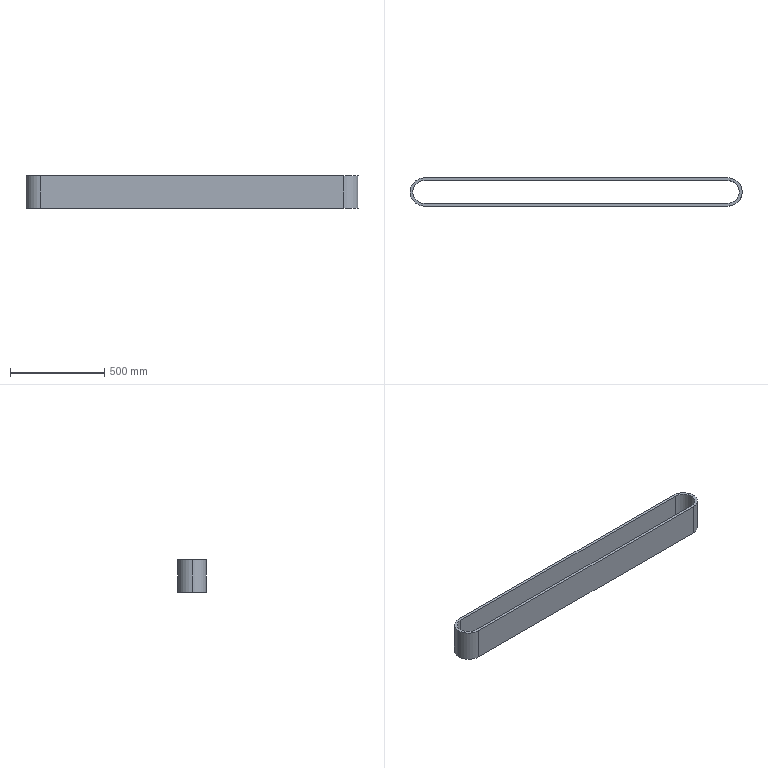Part | SolidWorks | features Extrusion 1 | 1 solid | 12 faces | box 1760 x 150 x 170 mm | volume 9292493 mm3 | cylinder 6 | plane 6 | commonest cylinder face diameters 120 x3 150 x3
STEP:
#1=CARTESIAN_POINT('',(-1610.,60.,170.));
#2=VERTEX_POINT('',#1);
#3=CARTESIAN_POINT('',(-1670.,0.,170.));
#4=VERTEX_POINT('',#3);
#5=CARTESIAN_POINT('',(-1610.,0.,170.));
#6=DIRECTION('',(0.,0.,1.));
#7=DIRECTION('',(1.,0.,0.));
#8=AXIS2_PLACEMENT_3D('',#5,#6,#7);
#9=CIRCLE('',#8,60.);
#10=EDGE_CURVE('',#2,#4,#9,.T.);
#11=ORIENTED_EDGE('',*,*,#10,.T.);
#12=CARTESIAN_POINT('',(-1670.,0.,0.));
#13=VERTEX_POINT('',#12);
#14=CARTESIAN_POINT('',(-1670.,0.,170.));
#15=DIRECTION('',(0.,0.,-1.));
#16=VECTOR('',#15,1000.);
#17=LINE('',#14,#16);
#18=EDGE_CURVE('',#4,#13,#17,.T.);
#19=ORIENTED_EDGE('',*,*,#18,.T.);
#20=CARTESIAN_POINT('',(-1610.,60.,0.));
#21=VERTEX_POINT('',#20);
#22=CARTESIAN_POINT('',(-1610.,0.,0.));
#23=DIRECTION('',(0.,0.,1.));
#24=DIRECTION('',(1.,0.,0.));
#25=AXIS2_PLACEMENT_3D('',#22,#23,#24);
#26=CIRCLE('',#25,60.);
#27=EDGE_CURVE('',#21,#13,#26,.T.);
#28=ORIENTED_EDGE('',*,*,#27,.F.);
#29=CARTESIAN_POINT('',(-1610.,60.,170.));
#30=DIRECTION('',(0.,0.,-1.));
#31=VECTOR('',#30,1000.);
#32=LINE('',#29,#31);
#33=EDGE_CURVE('',#2,#21,#32,.T.);
#34=ORIENTED_EDGE('',*,*,#33,.F.);
#35=EDGE_LOOP('',(#11,#19,#28,#34));
#36=FACE_OUTER_BOUND('',#35,.T.);
#37=CARTESIAN_POINT('',(-1610.,0.,170.));
#38=DIRECTION('',(0.,0.,-1.));
#39=DIRECTION('',(-1.,0.,0.));
#40=AXIS2_PLACEMENT_3D('',#37,#38,#39);
#41=CYLINDRICAL_SURFACE('',#40,60.);
#42=ADVANCED_FACE('',(#36),#41,.F.);
#43=CARTESIAN_POINT('',(-1685.,0.,170.));
#44=VERTEX_POINT('',#43);
#45=CARTESIAN_POINT('',(-1610.,-75.,170.));
#46=VERTEX_POINT('',#45);
#47=CARTESIAN_POINT('',(-1610.,0.,170.));
#48=DIRECTION('',(0.,0.,1.));
#49=DIRECTION('',(1.,0.,0.));
#50=AXIS2_PLACEMENT_3D('',#47,#48,#49);
#51=CIRCLE('',#50,75.);
#52=EDGE_CURVE('',#44,#46,#51,.T.);
#53=ORIENTED_EDGE('',*,*,#52,.F.);
#54=CARTESIAN_POINT('',(-1685.,0.,0.));
#55=VERTEX_POINT('',#54);
#56=CARTESIAN_POINT('',(-1685.,0.,170.));
#57=DIRECTION('',(0.,0.,-1.));
#58=VECTOR('',#57,1000.);
#59=LINE('',#56,#58);
#60=EDGE_CURVE('',#44,#55,#59,.T.);
#61=ORIENTED_EDGE('',*,*,#60,.T.);
#62=CARTESIAN_POINT('',(-1610.,-75.,0.));
#63=VERTEX_POINT('',#62);
#64=CARTESIAN_POINT('',(-1610.,0.,0.));
#65=DIRECTION('',(0.,0.,1.));
#66=DIRECTION('',(1.,0.,0.));
#67=AXIS2_PLACEMENT_3D('',#64,#65,#66);
#68=CIRCLE('',#67,75.);
#69=EDGE_CURVE('',#55,#63,#68,.T.);
#70=ORIENTED_EDGE('',*,*,#69,.T.);
#71=CARTESIAN_POINT('',(-1610.,-75.,170.));
#72=DIRECTION('',(0.,0.,-1.));
#73=VECTOR('',#72,1000.);
#74=LINE('',#71,#73);
#75=EDGE_CURVE('',#46,#63,#74,.T.);
#76=ORIENTED_EDGE('',*,*,#75,.F.);
#77=EDGE_LOOP('',(#53,#61,#70,#76));
#78=FACE_OUTER_BOUND('',#77,.T.);
#79=CARTESIAN_POINT('',(-1610.,0.,170.));
#80=DIRECTION('',(0.,0.,-1.));
#81=DIRECTION('',(-1.,0.,0.));
#82=AXIS2_PLACEMENT_3D('',#79,#80,#81);
#83=CYLINDRICAL_SURFACE('',#82,75.);
#84=ADVANCED_FACE('',(#78),#83,.T.);
#85=CARTESIAN_POINT('',(0.,-75.,170.));
#86=VERTEX_POINT('',#85);
#87=CARTESIAN_POINT('',(0.,75.,170.));
#88=VERTEX_POINT('',#87);
#89=CARTESIAN_POINT('',(0.,0.,170.));
#90=DIRECTION('',(0.,0.,1.));
#91=DIRECTION('',(1.,0.,0.));
#92=AXIS2_PLACEMENT_3D('',#89,#90,#91);
#93=CIRCLE('',#92,75.);
#94=EDGE_CURVE('',#86,#88,#93,.T.);
#95=ORIENTED_EDGE('',*,*,#94,.T.);
#96=CARTESIAN_POINT('',(-1610.,75.,170.));
#97=VERTEX_POINT('',#96);
#98=CARTESIAN_POINT('',(0.,75.,170.));
#99=DIRECTION('',(-1.,0.,0.));
#100=VECTOR('',#99,1000.);
#101=LINE('',#98,#100);
#102=EDGE_CURVE('',#88,#97,#101,.T.);
#103=ORIENTED_EDGE('',*,*,#102,.T.);
#104=CARTESIAN_POINT('',(-1610.,0.,170.));
#105=DIRECTION('',(0.,0.,1.));
#106=DIRECTION('',(1.,0.,0.));
#107=AXIS2_PLACEMENT_3D('',#104,#105,#106);
#108=CIRCLE('',#107,75.);
#109=EDGE_CURVE('',#97,#44,#108,.T.);
#110=ORIENTED_EDGE('',*,*,#109,.T.);
#111=ORIENTED_EDGE('',*,*,#52,.T.);
#112=CARTESIAN_POINT('',(0.,-75.,170.));
#113=DIRECTION('',(1.,0.,0.));
#114=VECTOR('',#113,1000.);
#115=LINE('',#112,#114);
#116=EDGE_CURVE('',#46,#86,#115,.T.);
#117=ORIENTED_EDGE('',*,*,#116,.T.);
#118=EDGE_LOOP('',(#95,#103,#110,#111,#117));
#119=FACE_OUTER_BOUND('',#118,.T.);
#120=CARTESIAN_POINT('',(0.,60.,170.));
#121=VERTEX_POINT('',#120);
#122=CARTESIAN_POINT('',(0.,60.,170.));
#123=DIRECTION('',(-1.,0.,0.));
#124=VECTOR('',#123,1000.);
#125=LINE('',#122,#124);
#126=EDGE_CURVE('',#121,#2,#125,.T.);
#127=ORIENTED_EDGE('',*,*,#126,.F.);
#128=CARTESIAN_POINT('',(0.,-60.,170.));
#129=VERTEX_POINT('',#128);
#130=CARTESIAN_POINT('',(0.,0.,170.));
#131=DIRECTION('',(0.,0.,1.));
#132=DIRECTION('',(1.,0.,0.));
#133=AXIS2_PLACEMENT_3D('',#130,#131,#132);
#134=CIRCLE('',#133,60.);
#135=EDGE_CURVE('',#129,#121,#134,.T.);
#136=ORIENTED_EDGE('',*,*,#135,.F.);
#137=CARTESIAN_POINT('',(-1610.,-60.,170.));
#138=VERTEX_POINT('',#137);
#139=CARTESIAN_POINT('',(0.,-60.,170.));
#140=DIRECTION('',(1.,0.,0.));
#141=VECTOR('',#140,1000.);
#142=LINE('',#139,#141);
#143=EDGE_CURVE('',#138,#129,#142,.T.);
#144=ORIENTED_EDGE('',*,*,#143,.F.);
#145=CARTESIAN_POINT('',(-1610.,0.,170.));
#146=DIRECTION('',(0.,0.,1.));
#147=DIRECTION('',(1.,0.,0.));
#148=AXIS2_PLACEMENT_3D('',#145,#146,#147);
#149=CIRCLE('',#148,60.);
#150=EDGE_CURVE('',#4,#138,#149,.T.);
#151=ORIENTED_EDGE('',*,*,#150,.F.);
#152=ORIENTED_EDGE('',*,*,#10,.F.);
#153=EDGE_LOOP('',(#127,#136,#144,#151,#152));
#154=FACE_BOUND('',#153,.T.);
#155=CARTESIAN_POINT('',(0.,0.,170.));
#156=DIRECTION('',(0.,0.,1.));
#157=DIRECTION('',(1.,0.,0.));
#158=AXIS2_PLACEMENT_3D('',#155,#156,#157);
#159=PLANE('',#158);
#160=ADVANCED_FACE('',(#119,#154),#159,.T.);
#161=CARTESIAN_POINT('',(0.,-75.,0.));
#162=VERTEX_POINT('',#161);
#163=CARTESIAN_POINT('',(0.,75.,0.));
#164=VERTEX_POINT('',#163);
#165=CARTESIAN_POINT('',(0.,0.,0.));
#166=DIRECTION('',(0.,0.,1.));
#167=DIRECTION('',(1.,0.,0.));
#168=AXIS2_PLACEMENT_3D('',#165,#166,#167);
#169=CIRCLE('',#168,75.);
#170=EDGE_CURVE('',#162,#164,#169,.T.);
#171=ORIENTED_EDGE('',*,*,#170,.F.);
#172=CARTESIAN_POINT('',(0.,-75.,0.));
#173=DIRECTION('',(1.,0.,0.));
#174=VECTOR('',#173,1000.);
#175=LINE('',#172,#174);
#176=EDGE_CURVE('',#63,#162,#175,.T.);
#177=ORIENTED_EDGE('',*,*,#176,.F.);
#178=ORIENTED_EDGE('',*,*,#69,.F.);
#179=CARTESIAN_POINT('',(-1610.,75.,0.));
#180=VERTEX_POINT('',#179);
#181=CARTESIAN_POINT('',(-1610.,0.,0.));
#182=DIRECTION('',(0.,0.,1.));
#183=DIRECTION('',(1.,0.,0.));
#184=AXIS2_PLACEMENT_3D('',#181,#182,#183);
#185=CIRCLE('',#184,75.);
#186=EDGE_CURVE('',#180,#55,#185,.T.);
#187=ORIENTED_EDGE('',*,*,#186,.F.);
#188=CARTESIAN_POINT('',(0.,75.,0.));
#189=DIRECTION('',(-1.,0.,0.));
#190=VECTOR('',#189,1000.);
#191=LINE('',#188,#190);
#192=EDGE_CURVE('',#164,#180,#191,.T.);
#193=ORIENTED_EDGE('',*,*,#192,.F.);
#194=EDGE_LOOP('',(#171,#177,#178,#187,#193));
#195=FACE_OUTER_BOUND('',#194,.T.);
#196=CARTESIAN_POINT('',(0.,-60.,0.));
#197=VERTEX_POINT('',#196);
#198=CARTESIAN_POINT('',(0.,60.,0.));
#199=VERTEX_POINT('',#198);
#200=CARTESIAN_POINT('',(0.,0.,0.));
#201=DIRECTION('',(0.,0.,1.));
#202=DIRECTION('',(1.,0.,0.));
#203=AXIS2_PLACEMENT_3D('',#200,#201,#202);
#204=CIRCLE('',#203,60.);
#205=EDGE_CURVE('',#197,#199,#204,.T.);
#206=ORIENTED_EDGE('',*,*,#205,.T.);
#207=CARTESIAN_POINT('',(0.,60.,0.));
#208=DIRECTION('',(-1.,0.,0.));
#209=VECTOR('',#208,1000.);
#210=LINE('',#207,#209);
#211=EDGE_CURVE('',#199,#21,#210,.T.);
#212=ORIENTED_EDGE('',*,*,#211,.T.);
#213=ORIENTED_EDGE('',*,*,#27,.T.);
#214=CARTESIAN_POINT('',(-1610.,-60.,0.));
#215=VERTEX_POINT('',#214);
#216=CARTESIAN_POINT('',(-1610.,0.,0.));
#217=DIRECTION('',(0.,0.,1.));
#218=DIRECTION('',(1.,0.,0.));
#219=AXIS2_PLACEMENT_3D('',#216,#217,#218);
#220=CIRCLE('',#219,60.);
#221=EDGE_CURVE('',#13,#215,#220,.T.);
#222=ORIENTED_EDGE('',*,*,#221,.T.);
#223=CARTESIAN_POINT('',(0.,-60.,0.));
#224=DIRECTION('',(1.,0.,0.));
#225=VECTOR('',#224,1000.);
#226=LINE('',#223,#225);
#227=EDGE_CURVE('',#215,#197,#226,.T.);
#228=ORIENTED_EDGE('',*,*,#227,.T.);
#229=EDGE_LOOP('',(#206,#212,#213,#222,#228));
#230=FACE_BOUND('',#229,.T.);
#231=CARTESIAN_POINT('',(0.,0.,0.));
#232=DIRECTION('',(0.,0.,1.));
#233=DIRECTION('',(1.,0.,0.));
#234=AXIS2_PLACEMENT_3D('',#231,#232,#233);
#235=PLANE('',#234);
#236=ADVANCED_FACE('',(#195,#230),#235,.F.);
#237=ORIENTED_EDGE('',*,*,#170,.T.);
#238=CARTESIAN_POINT('',(0.,75.,170.));
#239=DIRECTION('',(0.,0.,-1.));
#240=VECTOR('',#239,1000.);
#241=LINE('',#238,#240);
#242=EDGE_CURVE('',#88,#164,#241,.T.);
#243=ORIENTED_EDGE('',*,*,#242,.F.);
#244=ORIENTED_EDGE('',*,*,#94,.F.);
#245=CARTESIAN_POINT('',(0.,-75.,170.));
#246=DIRECTION('',(0.,0.,-1.));
#247=VECTOR('',#246,1000.);
#248=LINE('',#245,#247);
#249=EDGE_CURVE('',#86,#162,#248,.T.);
#250=ORIENTED_EDGE('',*,*,#249,.T.);
#251=EDGE_LOOP('',(#237,#243,#244,#250));
#252=FACE_OUTER_BOUND('',#251,.T.);
#253=CARTESIAN_POINT('',(0.,0.,170.));
#254=DIRECTION('',(0.,0.,-1.));
#255=DIRECTION('',(-1.,0.,0.));
#256=AXIS2_PLACEMENT_3D('',#253,#254,#255);
#257=CYLINDRICAL_SURFACE('',#256,75.);
#258=ADVANCED_FACE('',(#252),#257,.T.);
#259=ORIENTED_EDGE('',*,*,#192,.T.);
#260=CARTESIAN_POINT('',(-1610.,75.,170.));
#261=DIRECTION('',(0.,0.,-1.));
#262=VECTOR('',#261,1000.);
#263=LINE('',#260,#262);
#264=EDGE_CURVE('',#97,#180,#263,.T.);
#265=ORIENTED_EDGE('',*,*,#264,.F.);
#266=ORIENTED_EDGE('',*,*,#102,.F.);
#267=ORIENTED_EDGE('',*,*,#242,.T.);
#268=EDGE_LOOP('',(#259,#265,#266,#267));
#269=FACE_OUTER_BOUND('',#268,.T.);
#270=CARTESIAN_POINT('',(0.,75.,170.));
#271=DIRECTION('',(0.,-1.,0.));
#272=DIRECTION('',(1.,0.,0.));
#273=AXIS2_PLACEMENT_3D('',#270,#271,#272);
#274=PLANE('',#273);
#275=ADVANCED_FACE('',(#269),#274,.F.);
#276=ORIENTED_EDGE('',*,*,#60,.F.);
#277=ORIENTED_EDGE('',*,*,#109,.F.);
#278=ORIENTED_EDGE('',*,*,#264,.T.);
#279=ORIENTED_EDGE('',*,*,#186,.T.);
#280=EDGE_LOOP('',(#276,#277,#278,#279));
#281=FACE_OUTER_BOUND('',#280,.T.);
#282=CARTESIAN_POINT('',(-1610.,0.,170.));
#283=DIRECTION('',(0.,0.,-1.));
#284=DIRECTION('',(-1.,0.,0.));
#285=AXIS2_PLACEMENT_3D('',#282,#283,#284);
#286=CYLINDRICAL_SURFACE('',#285,75.);
#287=ADVANCED_FACE('',(#281),#286,.T.);
#288=ORIENTED_EDGE('',*,*,#176,.T.);
#289=ORIENTED_EDGE('',*,*,#249,.F.);
#290=ORIENTED_EDGE('',*,*,#116,.F.);
#291=ORIENTED_EDGE('',*,*,#75,.T.);
#292=EDGE_LOOP('',(#288,#289,#290,#291));
#293=FACE_OUTER_BOUND('',#292,.T.);
#294=CARTESIAN_POINT('',(0.,-75.,170.));
#295=DIRECTION('',(0.,1.,0.));
#296=DIRECTION('',(-1.,0.,0.));
#297=AXIS2_PLACEMENT_3D('',#294,#295,#296);
#298=PLANE('',#297);
#299=ADVANCED_FACE('',(#293),#298,.F.);
#300=ORIENTED_EDGE('',*,*,#205,.F.);
#301=CARTESIAN_POINT('',(0.,-60.,170.));
#302=DIRECTION('',(0.,0.,-1.));
#303=VECTOR('',#302,1000.);
#304=LINE('',#301,#303);
#305=EDGE_CURVE('',#129,#197,#304,.T.);
#306=ORIENTED_EDGE('',*,*,#305,.F.);
#307=ORIENTED_EDGE('',*,*,#135,.T.);
#308=CARTESIAN_POINT('',(0.,60.,170.));
#309=DIRECTION('',(0.,0.,-1.));
#310=VECTOR('',#309,1000.);
#311=LINE('',#308,#310);
#312=EDGE_CURVE('',#121,#199,#311,.T.);
#313=ORIENTED_EDGE('',*,*,#312,.T.);
#314=EDGE_LOOP('',(#300,#306,#307,#313));
#315=FACE_OUTER_BOUND('',#314,.T.);
#316=CARTESIAN_POINT('',(0.,0.,170.));
#317=DIRECTION('',(0.,0.,-1.));
#318=DIRECTION('',(-1.,0.,0.));
#319=AXIS2_PLACEMENT_3D('',#316,#317,#318);
#320=CYLINDRICAL_SURFACE('',#319,60.);
#321=ADVANCED_FACE('',(#315),#320,.F.);
#322=ORIENTED_EDGE('',*,*,#211,.F.);
#323=ORIENTED_EDGE('',*,*,#312,.F.);
#324=ORIENTED_EDGE('',*,*,#126,.T.);
#325=ORIENTED_EDGE('',*,*,#33,.T.);
#326=EDGE_LOOP('',(#322,#323,#324,#325));
#327=FACE_OUTER_BOUND('',#326,.T.);
#328=CARTESIAN_POINT('',(0.,60.,170.));
#329=DIRECTION('',(0.,-1.,0.));
#330=DIRECTION('',(1.,0.,0.));
#331=AXIS2_PLACEMENT_3D('',#328,#329,#330);
#332=PLANE('',#331);
#333=ADVANCED_FACE('',(#327),#332,.T.);
#334=ORIENTED_EDGE('',*,*,#18,.F.);
#335=ORIENTED_EDGE('',*,*,#150,.T.);
#336=CARTESIAN_POINT('',(-1610.,-60.,170.));
#337=DIRECTION('',(0.,0.,-1.));
#338=VECTOR('',#337,1000.);
#339=LINE('',#336,#338);
#340=EDGE_CURVE('',#138,#215,#339,.T.);
#341=ORIENTED_EDGE('',*,*,#340,.T.);
#342=ORIENTED_EDGE('',*,*,#221,.F.);
#343=EDGE_LOOP('',(#334,#335,#341,#342));
#344=FACE_OUTER_BOUND('',#343,.T.);
#345=CARTESIAN_POINT('',(-1610.,0.,170.));
#346=DIRECTION('',(0.,0.,-1.));
#347=DIRECTION('',(-1.,0.,0.));
#348=AXIS2_PLACEMENT_3D('',#345,#346,#347);
#349=CYLINDRICAL_SURFACE('',#348,60.);
#350=ADVANCED_FACE('',(#344),#349,.F.);
#351=ORIENTED_EDGE('',*,*,#227,.F.);
#352=ORIENTED_EDGE('',*,*,#340,.F.);
#353=ORIENTED_EDGE('',*,*,#143,.T.);
#354=ORIENTED_EDGE('',*,*,#305,.T.);
#355=EDGE_LOOP('',(#351,#352,#353,#354));
#356=FACE_OUTER_BOUND('',#355,.T.);
#357=CARTESIAN_POINT('',(0.,-60.,170.));
#358=DIRECTION('',(0.,1.,0.));
#359=DIRECTION('',(-1.,0.,0.));
#360=AXIS2_PLACEMENT_3D('',#357,#358,#359);
#361=PLANE('',#360);
#362=ADVANCED_FACE('',(#356),#361,.T.);
#363=CLOSED_SHELL('',(#42,#84,#160,#236,#258,#275,#287,#299,#321,#333,#350,#362));
#364=MANIFOLD_SOLID_BREP('',#363);
#365=CARTESIAN_POINT('',(0.,0.,0.));
#366=DIRECTION('',(0.,0.,1.));
#367=DIRECTION('',(1.,0.,0.));
#368=AXIS2_PLACEMENT_3D('',#365,#366,#367);
#369=(LENGTH_UNIT()NAMED_UNIT(*)SI_UNIT(.MILLI.,.METRE.));
#370=UNCERTAINTY_MEASURE_WITH_UNIT(LENGTH_MEASURE(0.00001),#369,'','');
#371=(NAMED_UNIT(*)PLANE_ANGLE_UNIT()SI_UNIT($,.RADIAN.));
#372=(NAMED_UNIT(*)SI_UNIT($,.STERADIAN.)SOLID_ANGLE_UNIT());
#373=(GEOMETRIC_REPRESENTATION_CONTEXT(3)GLOBAL_UNCERTAINTY_ASSIGNED_CONTEXT((#370))GLOBAL_UNIT_ASSIGNED_CONTEXT((#369,#371,#372))REPRESENTATION_CONTEXT('',''));
#374=ADVANCED_BREP_SHAPE_REPRESENTATION('',(#364,#368),#373);